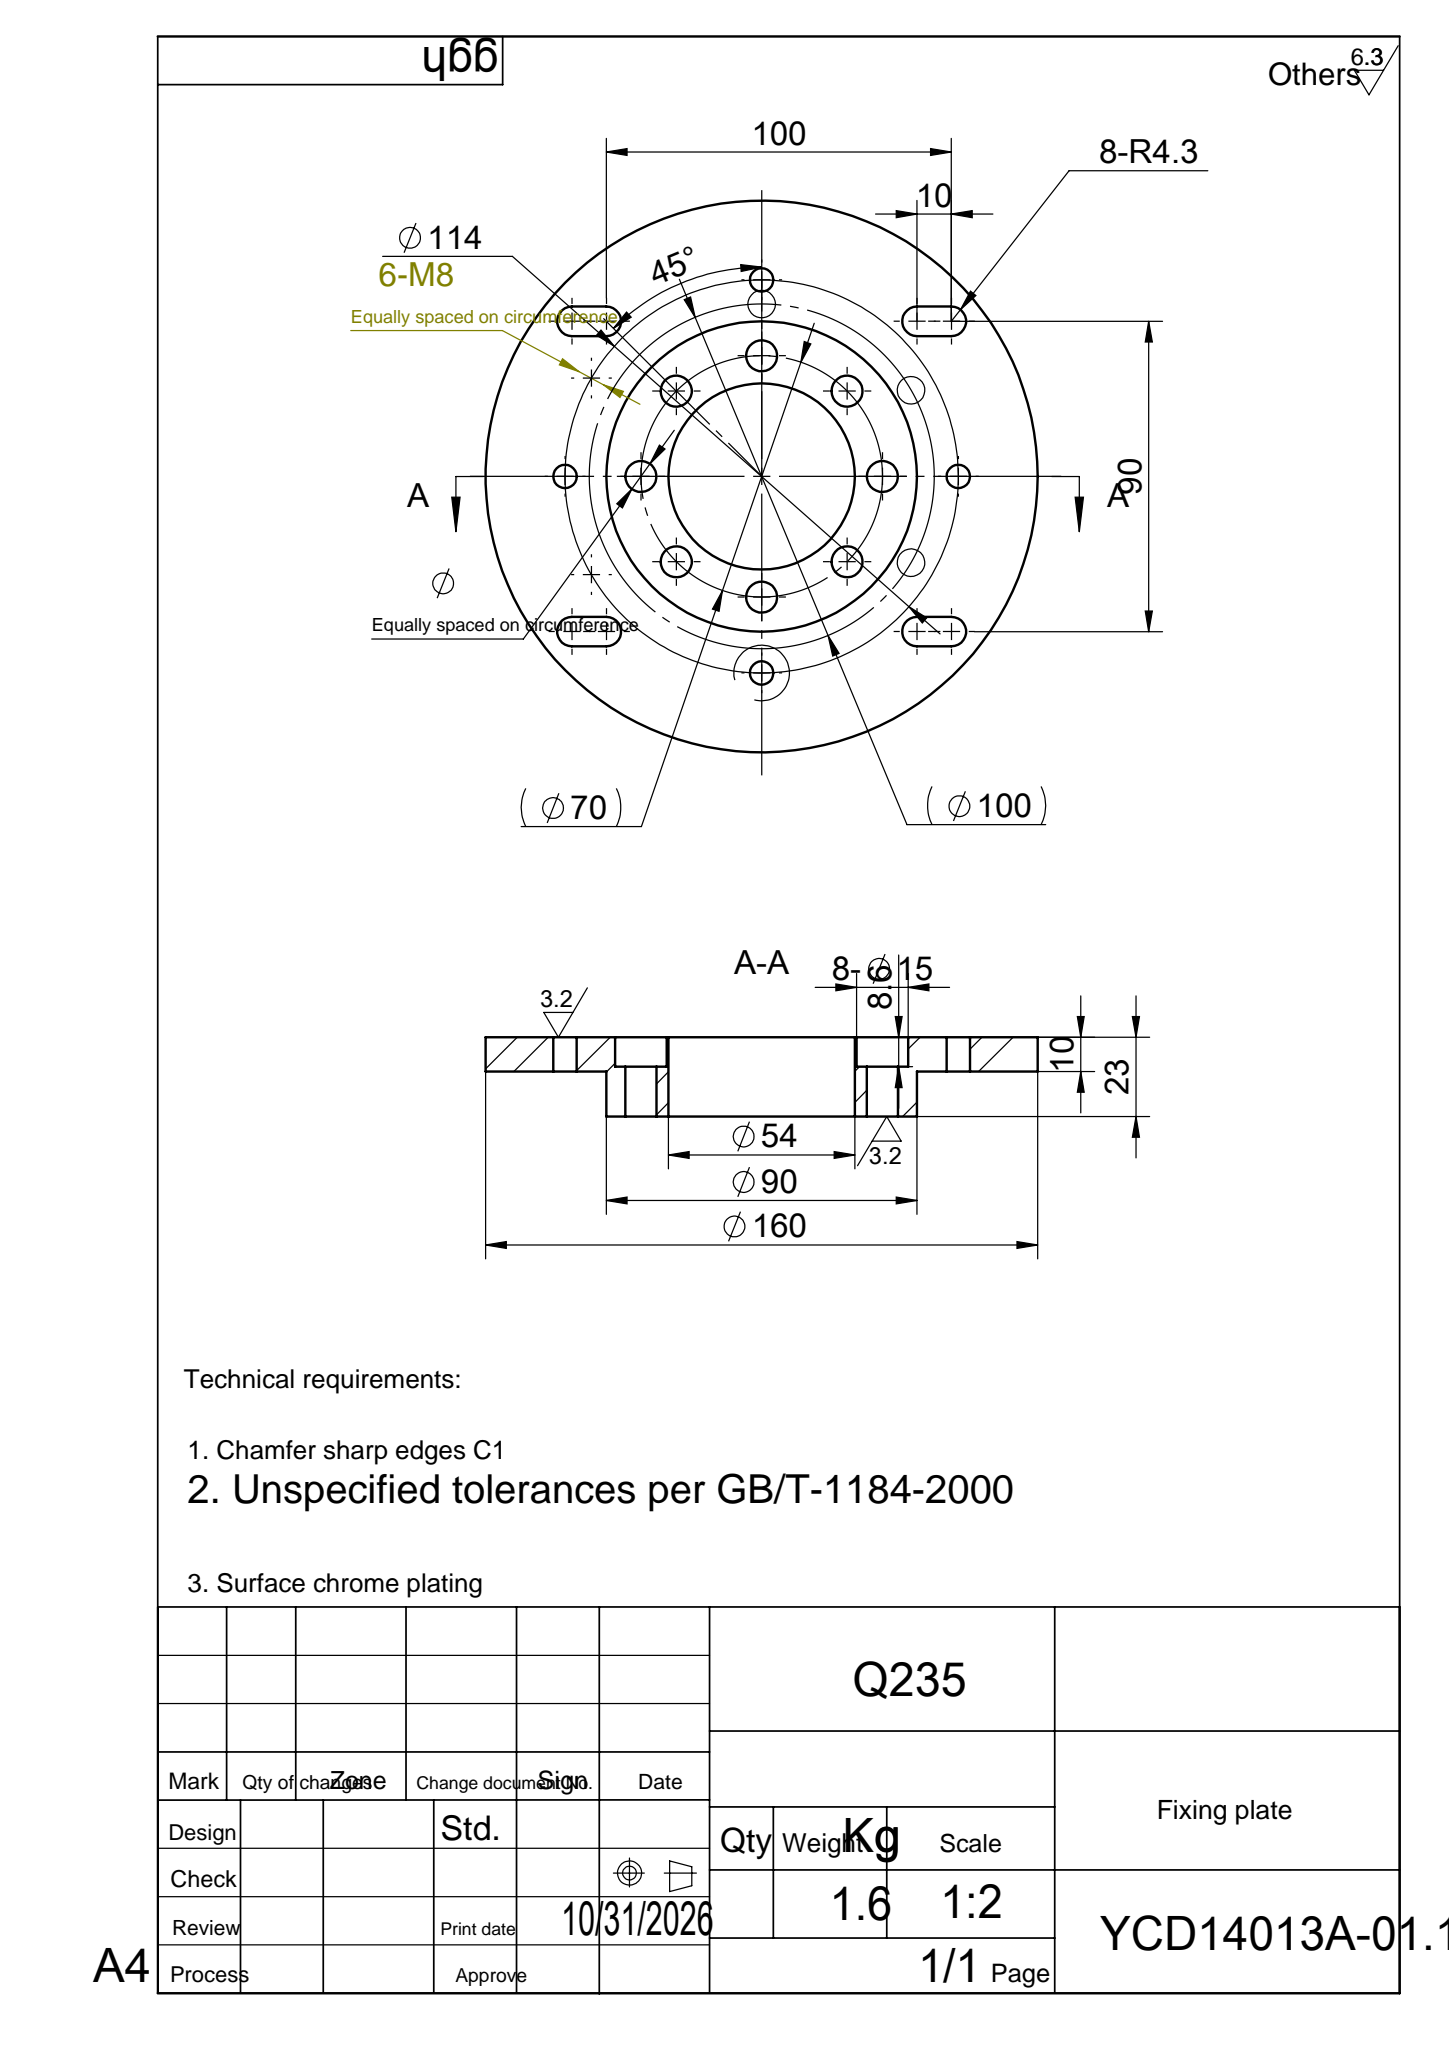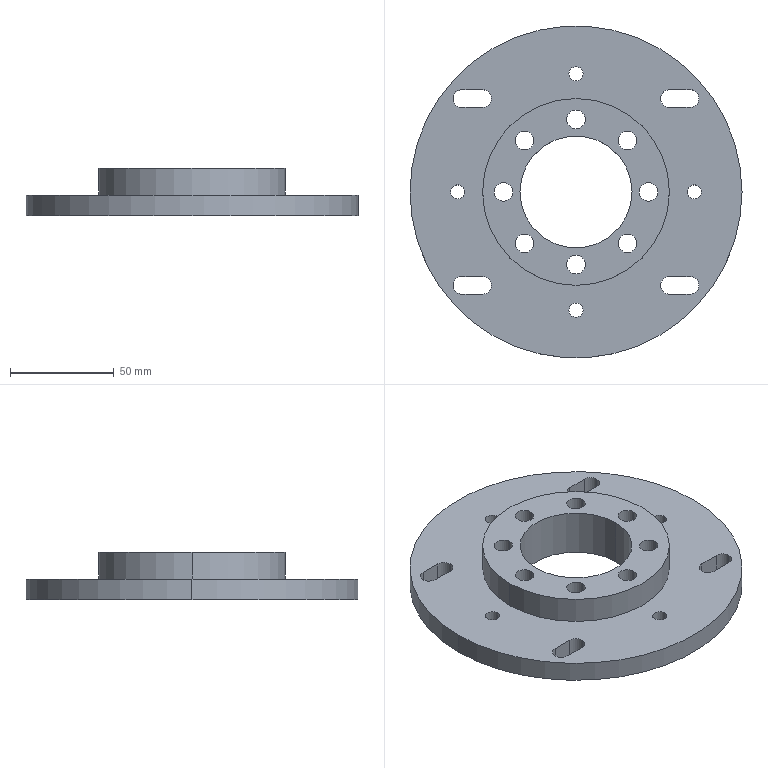Part | SolidWorks | features ICE 3, CirPattern 2, HoleWzd 2, Extrusion 1 | 1 solid | 77 faces | box 160 x 160 x 23 mm | volume 204439 mm3 | cylinder 58 | plane 19 | commonest cylinder face diameters 9 x16 15 x16 8.544 x12 6.8 x8 54 x2 90 x2